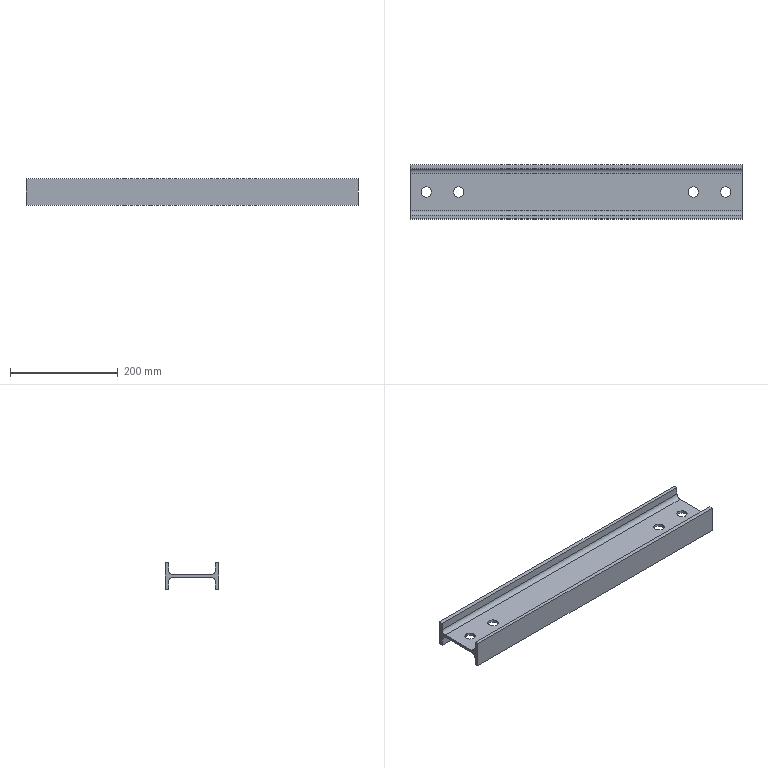Part | STEP file | Powder bin secondary beam 17 body_Default<As Machined> | 1 solid | 26 faces | box 615 x 100 x 50 mm | volume 723066 mm3 | plane 14 | cylinder 12 | commonest cylinder face diameters 19 x8 16 x4